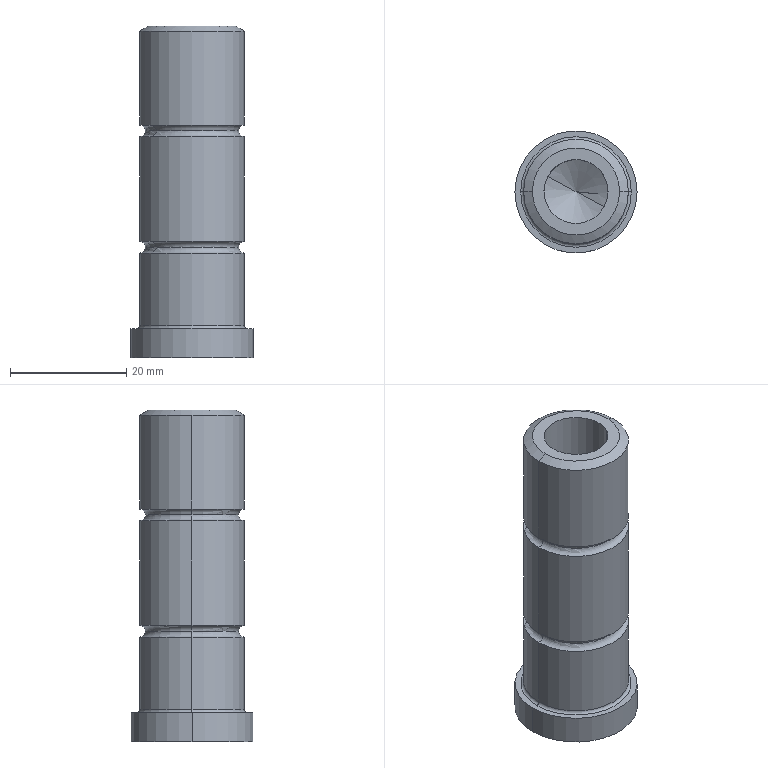Part | CATIA | 1 solid | 27 faces | box 21 x 21 x 57 mm | volume 12762 mm3 | cylinder 10 | torus 10 | cone 4 | plane 3 | commonest cylinder face diameters 18 x6 11 x2 21 x2
STEP:
#1=CARTESIAN_POINT('',(10.5,0.,-5.));
#2=VERTEX_POINT('',#1);
#3=CARTESIAN_POINT('',(-10.5,0.,-5.));
#4=VERTEX_POINT('',#3);
#5=CARTESIAN_POINT('',(0.,0.,-5.));
#6=DIRECTION('',(0.,0.,-1.));
#7=AXIS2_PLACEMENT_3D('',#5,#6,$);
#8=CIRCLE('',#7,10.5);
#9=EDGE_CURVE('',#2,#4,#8,.T.);
#10=ORIENTED_EDGE('',*,*,#9,.T.);
#11=CARTESIAN_POINT('',(0.,0.,-5.));
#12=DIRECTION('',(0.,0.,-1.));
#13=AXIS2_PLACEMENT_3D('',#11,#12,$);
#14=CIRCLE('',#13,10.5);
#15=EDGE_CURVE('',#4,#2,#14,.T.);
#16=ORIENTED_EDGE('',*,*,#15,.T.);
#17=EDGE_LOOP('',(#10,#16));
#18=FACE_OUTER_BOUND('',#17,.T.);
#19=CARTESIAN_POINT('',(0.,0.,-5.));
#20=DIRECTION('',(0.,0.,-1.));
#21=DIRECTION('',(1.,0.,0.));
#22=AXIS2_PLACEMENT_3D('',#19,#20,#21);
#23=PLANE('',#22);
#24=ADVANCED_FACE('',(#18),#23,.T.);
#25=CARTESIAN_POINT('',(-10.5,0.,0.));
#26=VERTEX_POINT('',#25);
#27=CARTESIAN_POINT('',(-10.5,0.,-2.5));
#28=DIRECTION('',(0.,0.,-1.));
#29=VECTOR('',#28,1.);
#30=LINE('',#27,#29);
#31=EDGE_CURVE('',#26,#4,#30,.T.);
#32=ORIENTED_EDGE('',*,*,#31,.F.);
#33=CARTESIAN_POINT('',(10.5,0.,0.));
#34=VERTEX_POINT('',#33);
#35=CARTESIAN_POINT('',(0.,0.,0.));
#36=DIRECTION('',(0.,0.,-1.));
#37=AXIS2_PLACEMENT_3D('',#35,#36,$);
#38=CIRCLE('',#37,10.5);
#39=EDGE_CURVE('',#26,#34,#38,.T.);
#40=ORIENTED_EDGE('',*,*,#39,.T.);
#41=CARTESIAN_POINT('',(10.5,0.,-2.5));
#42=DIRECTION('',(0.,0.,-1.));
#43=VECTOR('',#42,1.);
#44=LINE('',#41,#43);
#45=EDGE_CURVE('',#34,#2,#44,.T.);
#46=ORIENTED_EDGE('',*,*,#45,.T.);
#47=ORIENTED_EDGE('',*,*,#15,.F.);
#48=EDGE_LOOP('',(#32,#40,#46,#47));
#49=FACE_OUTER_BOUND('',#48,.T.);
#50=CARTESIAN_POINT('',(0.,0.,-2.5));
#51=DIRECTION('',(0.,0.,-1.));
#52=DIRECTION('',(1.,0.,0.));
#53=AXIS2_PLACEMENT_3D('',#50,#51,#52);
#54=CYLINDRICAL_SURFACE('',#53,10.5);
#55=ADVANCED_FACE('',(#49),#54,.T.);
#56=ORIENTED_EDGE('',*,*,#45,.F.);
#57=CARTESIAN_POINT('',(0.,0.,0.));
#58=DIRECTION('',(0.,0.,-1.));
#59=AXIS2_PLACEMENT_3D('',#57,#58,$);
#60=CIRCLE('',#59,10.5);
#61=EDGE_CURVE('',#34,#26,#60,.T.);
#62=ORIENTED_EDGE('',*,*,#61,.T.);
#63=ORIENTED_EDGE('',*,*,#31,.T.);
#64=ORIENTED_EDGE('',*,*,#9,.F.);
#65=EDGE_LOOP('',(#56,#62,#63,#64));
#66=FACE_OUTER_BOUND('',#65,.T.);
#67=ADVANCED_FACE('',(#66),#54,.T.);
#68=CARTESIAN_POINT('',(0.,0.,28.825));
#69=VERTEX_POINT('',#68);
#70=CARTESIAN_POINT('',(-4.827,2.637,32.));
#71=VERTEX_POINT('',#70);
#72=CARTESIAN_POINT('',(-2.413,1.318,30.412));
#73=DIRECTION('',(-0.76,0.4152,0.5));
#74=VECTOR('',#73,1.);
#75=LINE('',#72,#74);
#76=EDGE_CURVE('',#69,#71,#75,.T.);
#77=ORIENTED_EDGE('',*,*,#76,.T.);
#78=CARTESIAN_POINT('',(4.827,-2.637,32.));
#79=VERTEX_POINT('',#78);
#80=CARTESIAN_POINT('',(0.,0.,32.));
#81=DIRECTION('',(0.,0.,1.));
#82=AXIS2_PLACEMENT_3D('',#80,#81,$);
#83=CIRCLE('',#82,5.5);
#84=EDGE_CURVE('',#79,#71,#83,.F.);
#85=ORIENTED_EDGE('',*,*,#84,.F.);
#86=CARTESIAN_POINT('',(2.413,-1.318,30.412));
#87=DIRECTION('',(0.76,-0.4152,0.5));
#88=VECTOR('',#87,1.);
#89=LINE('',#86,#88);
#90=EDGE_CURVE('',#69,#79,#89,.T.);
#91=ORIENTED_EDGE('',*,*,#90,.F.);
#92=EDGE_LOOP('',(#77,#85,#91));
#93=FACE_OUTER_BOUND('',#92,.T.);
#94=CARTESIAN_POINT('',(0.,0.,28.825));
#95=DIRECTION('',(0.,0.,1.));
#96=DIRECTION('',(0.8776,-0.4794,0.));
#97=AXIS2_PLACEMENT_3D('',#94,#95,#96);
#98=CONICAL_SURFACE('',#97,0.,1.047);
#99=ADVANCED_FACE('',(#93),#98,.F.);
#100=ORIENTED_EDGE('',*,*,#90,.T.);
#101=CARTESIAN_POINT('',(0.,0.,32.));
#102=DIRECTION('',(0.,0.,1.));
#103=AXIS2_PLACEMENT_3D('',#101,#102,$);
#104=CIRCLE('',#103,5.5);
#105=EDGE_CURVE('',#71,#79,#104,.F.);
#106=ORIENTED_EDGE('',*,*,#105,.F.);
#107=ORIENTED_EDGE('',*,*,#76,.F.);
#108=EDGE_LOOP('',(#100,#106,#107));
#109=FACE_OUTER_BOUND('',#108,.T.);
#110=ADVANCED_FACE('',(#109),#98,.F.);
#111=CARTESIAN_POINT('',(-4.827,2.637,52.));
#112=VERTEX_POINT('',#111);
#113=CARTESIAN_POINT('',(4.827,-2.637,52.));
#114=VERTEX_POINT('',#113);
#115=CARTESIAN_POINT('',(0.,0.,52.));
#116=DIRECTION('',(0.,0.,-1.));
#117=AXIS2_PLACEMENT_3D('',#115,#116,$);
#118=CIRCLE('',#117,5.5);
#119=EDGE_CURVE('',#112,#114,#118,.F.);
#120=ORIENTED_EDGE('',*,*,#119,.T.);
#121=CARTESIAN_POINT('',(4.827,-2.637,42.155));
#122=DIRECTION('',(0.,0.,-1.));
#123=VECTOR('',#122,1.);
#124=LINE('',#121,#123);
#125=EDGE_CURVE('',#79,#114,#124,.F.);
#126=ORIENTED_EDGE('',*,*,#125,.F.);
#127=ORIENTED_EDGE('',*,*,#84,.T.);
#128=CARTESIAN_POINT('',(-4.827,2.637,42.155));
#129=DIRECTION('',(0.,0.,-1.));
#130=VECTOR('',#129,1.);
#131=LINE('',#128,#130);
#132=EDGE_CURVE('',#71,#112,#131,.F.);
#133=ORIENTED_EDGE('',*,*,#132,.T.);
#134=EDGE_LOOP('',(#120,#126,#127,#133));
#135=FACE_OUTER_BOUND('',#134,.T.);
#136=CARTESIAN_POINT('',(0.,0.,51.9));
#137=DIRECTION('',(0.,0.,-1.));
#138=DIRECTION('',(0.8776,-0.4794,0.));
#139=AXIS2_PLACEMENT_3D('',#136,#137,#138);
#140=CYLINDRICAL_SURFACE('',#139,5.5);
#141=ADVANCED_FACE('',(#135),#140,.F.);
#142=CARTESIAN_POINT('',(0.,0.,52.));
#143=DIRECTION('',(0.,0.,-1.));
#144=AXIS2_PLACEMENT_3D('',#142,#143,$);
#145=CIRCLE('',#144,5.5);
#146=EDGE_CURVE('',#114,#112,#145,.F.);
#147=ORIENTED_EDGE('',*,*,#146,.T.);
#148=ORIENTED_EDGE('',*,*,#132,.F.);
#149=ORIENTED_EDGE('',*,*,#105,.T.);
#150=ORIENTED_EDGE('',*,*,#125,.T.);
#151=EDGE_LOOP('',(#147,#148,#149,#150));
#152=FACE_OUTER_BOUND('',#151,.T.);
#153=ADVANCED_FACE('',(#152),#140,.F.);
#154=CARTESIAN_POINT('',(-7.5,0.000000168,52.));
#155=VERTEX_POINT('',#154);
#156=CARTESIAN_POINT('',(7.5,0.,52.));
#157=VERTEX_POINT('',#156);
#158=CARTESIAN_POINT('',(0.,0.,52.));
#159=DIRECTION('',(0.,0.,1.));
#160=AXIS2_PLACEMENT_3D('',#158,#159,$);
#161=CIRCLE('',#160,7.5);
#162=EDGE_CURVE('',#155,#157,#161,.T.);
#163=ORIENTED_EDGE('',*,*,#162,.T.);
#164=CARTESIAN_POINT('',(0.,0.,52.));
#165=DIRECTION('',(0.,0.,1.));
#166=AXIS2_PLACEMENT_3D('',#164,#165,$);
#167=CIRCLE('',#166,7.5);
#168=EDGE_CURVE('',#157,#155,#167,.T.);
#169=ORIENTED_EDGE('',*,*,#168,.T.);
#170=EDGE_LOOP('',(#163,#169));
#171=FACE_OUTER_BOUND('',#170,.T.);
#172=ORIENTED_EDGE('',*,*,#119,.F.);
#173=ORIENTED_EDGE('',*,*,#146,.F.);
#174=EDGE_LOOP('',(#172,#173));
#175=FACE_BOUND('',#174,.T.);
#176=CARTESIAN_POINT('',(0.,0.,52.));
#177=DIRECTION('',(0.,0.,1.));
#178=DIRECTION('',(1.,0.,0.));
#179=AXIS2_PLACEMENT_3D('',#176,#177,#178);
#180=PLANE('',#179);
#181=ADVANCED_FACE('',(#171,#175),#180,.T.);
#182=CARTESIAN_POINT('',(-9.,0.,51.134));
#183=VERTEX_POINT('',#182);
#184=CARTESIAN_POINT('',(-8.25,0.,51.567));
#185=DIRECTION('',(-0.866,0.,-0.5));
#186=VECTOR('',#185,1.);
#187=LINE('',#184,#186);
#188=EDGE_CURVE('',#155,#183,#187,.T.);
#189=ORIENTED_EDGE('',*,*,#188,.T.);
#190=CARTESIAN_POINT('',(9.,0.,51.134));
#191=VERTEX_POINT('',#190);
#192=CARTESIAN_POINT('',(0.,0.,51.134));
#193=DIRECTION('',(0.,0.,1.));
#194=AXIS2_PLACEMENT_3D('',#192,#193,$);
#195=CIRCLE('',#194,9.);
#196=EDGE_CURVE('',#183,#191,#195,.T.);
#197=ORIENTED_EDGE('',*,*,#196,.T.);
#198=CARTESIAN_POINT('',(8.25,0.,51.567));
#199=DIRECTION('',(0.866,0.,-0.5));
#200=VECTOR('',#199,1.);
#201=LINE('',#198,#200);
#202=EDGE_CURVE('',#157,#191,#201,.T.);
#203=ORIENTED_EDGE('',*,*,#202,.F.);
#204=ORIENTED_EDGE('',*,*,#162,.F.);
#205=EDGE_LOOP('',(#189,#197,#203,#204));
#206=FACE_OUTER_BOUND('',#205,.T.);
#207=CARTESIAN_POINT('',(0.,0.,56.33));
#208=DIRECTION('',(0.,0.,-1.));
#209=DIRECTION('',(-0.894,0.4481,0.));
#210=AXIS2_PLACEMENT_3D('',#207,#208,#209);
#211=CONICAL_SURFACE('',#210,0.,1.047);
#212=ADVANCED_FACE('',(#206),#211,.T.);
#213=ORIENTED_EDGE('',*,*,#202,.T.);
#214=CARTESIAN_POINT('',(0.,0.,51.134));
#215=DIRECTION('',(0.,0.,1.));
#216=AXIS2_PLACEMENT_3D('',#214,#215,$);
#217=CIRCLE('',#216,9.);
#218=EDGE_CURVE('',#191,#183,#217,.T.);
#219=ORIENTED_EDGE('',*,*,#218,.T.);
#220=ORIENTED_EDGE('',*,*,#188,.F.);
#221=ORIENTED_EDGE('',*,*,#168,.F.);
#222=EDGE_LOOP('',(#213,#219,#220,#221));
#223=FACE_OUTER_BOUND('',#222,.T.);
#224=CARTESIAN_POINT('',(0.,0.,56.33));
#225=DIRECTION('',(0.,0.,-1.));
#226=DIRECTION('',(1.,0.,0.));
#227=AXIS2_PLACEMENT_3D('',#224,#225,#226);
#228=CONICAL_SURFACE('',#227,0.,1.047);
#229=ADVANCED_FACE('',(#223),#228,.T.);
#230=ORIENTED_EDGE('',*,*,#39,.F.);
#231=ORIENTED_EDGE('',*,*,#61,.F.);
#232=EDGE_LOOP('',(#230,#231));
#233=FACE_OUTER_BOUND('',#232,.T.);
#234=CARTESIAN_POINT('',(9.5,0.,0.));
#235=VERTEX_POINT('',#234);
#236=CARTESIAN_POINT('',(-9.5,-0.000000008,0.));
#237=VERTEX_POINT('',#236);
#238=CARTESIAN_POINT('',(0.,0.,0.));
#239=DIRECTION('',(0.,0.,1.));
#240=AXIS2_PLACEMENT_3D('',#238,#239,$);
#241=CIRCLE('',#240,9.5);
#242=EDGE_CURVE('',#235,#237,#241,.F.);
#243=ORIENTED_EDGE('',*,*,#242,.T.);
#244=CARTESIAN_POINT('',(0.,0.,0.));
#245=DIRECTION('',(0.,0.,1.));
#246=AXIS2_PLACEMENT_3D('',#244,#245,$);
#247=CIRCLE('',#246,9.5);
#248=EDGE_CURVE('',#237,#235,#247,.F.);
#249=ORIENTED_EDGE('',*,*,#248,.T.);
#250=EDGE_LOOP('',(#243,#249));
#251=FACE_BOUND('',#250,.T.);
#252=CARTESIAN_POINT('',(0.,0.,0.));
#253=DIRECTION('',(0.,0.,1.));
#254=DIRECTION('',(1.,0.,0.));
#255=AXIS2_PLACEMENT_3D('',#252,#253,#254);
#256=PLANE('',#255);
#257=ADVANCED_FACE('',(#233,#251),#256,.T.);
#258=CARTESIAN_POINT('',(-9.,0.,0.5));
#259=VERTEX_POINT('',#258);
#260=CARTESIAN_POINT('',(9.,0.,0.5));
#261=VERTEX_POINT('',#260);
#262=CARTESIAN_POINT('',(0.,0.,0.5));
#263=DIRECTION('',(0.,0.,1.));
#264=AXIS2_PLACEMENT_3D('',#262,#263,$);
#265=CIRCLE('',#264,9.);
#266=EDGE_CURVE('',#259,#261,#265,.F.);
#267=ORIENTED_EDGE('',*,*,#266,.T.);
#268=CARTESIAN_POINT('',(9.5,0.,0.5));
#269=DIRECTION('',(0.,-1.,0.));
#270=AXIS2_PLACEMENT_3D('',#268,#269,$);
#271=CIRCLE('',#270,0.5);
#272=EDGE_CURVE('',#261,#235,#271,.T.);
#273=ORIENTED_EDGE('',*,*,#272,.T.);
#274=ORIENTED_EDGE('',*,*,#248,.F.);
#275=CARTESIAN_POINT('',(-9.5,0.000000067,0.5));
#276=DIRECTION('',(0.000000007,1.,0.));
#277=AXIS2_PLACEMENT_3D('',#275,#276,$);
#278=CIRCLE('',#277,0.5);
#279=EDGE_CURVE('',#259,#237,#278,.T.);
#280=ORIENTED_EDGE('',*,*,#279,.F.);
#281=EDGE_LOOP('',(#267,#273,#274,#280));
#282=FACE_OUTER_BOUND('',#281,.T.);
#283=CARTESIAN_POINT('',(0.,0.,0.5));
#284=DIRECTION('',(0.,0.,1.));
#285=DIRECTION('',(1.,0.,0.));
#286=AXIS2_PLACEMENT_3D('',#283,#284,#285);
#287=TOROIDAL_SURFACE('',#286,9.5,0.5);
#288=ADVANCED_FACE('',(#282),#287,.F.);
#289=CARTESIAN_POINT('',(0.,0.,0.5));
#290=DIRECTION('',(0.,0.,1.));
#291=AXIS2_PLACEMENT_3D('',#289,#290,$);
#292=CIRCLE('',#291,9.);
#293=EDGE_CURVE('',#261,#259,#292,.F.);
#294=ORIENTED_EDGE('',*,*,#293,.T.);
#295=ORIENTED_EDGE('',*,*,#279,.T.);
#296=ORIENTED_EDGE('',*,*,#242,.F.);
#297=ORIENTED_EDGE('',*,*,#272,.F.);
#298=EDGE_LOOP('',(#294,#295,#296,#297));
#299=FACE_OUTER_BOUND('',#298,.T.);
#300=CARTESIAN_POINT('',(0.,0.,0.5));
#301=DIRECTION('',(0.,0.,1.));
#302=DIRECTION('',(-0.9997,0.02353,0.));
#303=AXIS2_PLACEMENT_3D('',#300,#301,#302);
#304=TOROIDAL_SURFACE('',#303,9.5,0.5);
#305=ADVANCED_FACE('',(#299),#304,.F.);
#306=CARTESIAN_POINT('',(-9.,0.000000203,15.));
#307=VERTEX_POINT('',#306);
#308=CARTESIAN_POINT('',(-9.,0.,33.));
#309=VERTEX_POINT('',#308);
#310=CARTESIAN_POINT('',(-9.,0.,26.));
#311=DIRECTION('',(0.,0.,1.));
#312=VECTOR('',#311,1.);
#313=LINE('',#310,#312);
#314=EDGE_CURVE('',#307,#309,#313,.T.);
#315=ORIENTED_EDGE('',*,*,#314,.T.);
#316=CARTESIAN_POINT('',(9.,0.,33.));
#317=VERTEX_POINT('',#316);
#318=CARTESIAN_POINT('',(0.,0.,33.));
#319=DIRECTION('',(0.,0.,1.));
#320=AXIS2_PLACEMENT_3D('',#318,#319,$);
#321=CIRCLE('',#320,9.);
#322=EDGE_CURVE('',#317,#309,#321,.T.);
#323=ORIENTED_EDGE('',*,*,#322,.F.);
#324=CARTESIAN_POINT('',(9.,-0.000000009,15.));
#325=VERTEX_POINT('',#324);
#326=CARTESIAN_POINT('',(9.,0.,26.));
#327=DIRECTION('',(0.,0.,1.));
#328=VECTOR('',#327,1.);
#329=LINE('',#326,#328);
#330=EDGE_CURVE('',#325,#317,#329,.T.);
#331=ORIENTED_EDGE('',*,*,#330,.F.);
#332=CARTESIAN_POINT('',(0.,0.,15.));
#333=DIRECTION('',(0.,0.,1.));
#334=AXIS2_PLACEMENT_3D('',#332,#333,$);
#335=CIRCLE('',#334,9.);
#336=EDGE_CURVE('',#325,#307,#335,.T.);
#337=ORIENTED_EDGE('',*,*,#336,.T.);
#338=EDGE_LOOP('',(#315,#323,#331,#337));
#339=FACE_OUTER_BOUND('',#338,.T.);
#340=CARTESIAN_POINT('',(0.,0.,26.));
#341=DIRECTION('',(0.,0.,1.));
#342=DIRECTION('',(1.,0.,0.));
#343=AXIS2_PLACEMENT_3D('',#340,#341,#342);
#344=CYLINDRICAL_SURFACE('',#343,9.);
#345=ADVANCED_FACE('',(#339),#344,.T.);
#346=CARTESIAN_POINT('',(9.,0.,13.));
#347=VERTEX_POINT('',#346);
#348=CARTESIAN_POINT('',(9.,0.,26.));
#349=DIRECTION('',(0.,0.,1.));
#350=VECTOR('',#349,1.);
#351=LINE('',#348,#350);
#352=EDGE_CURVE('',#261,#347,#351,.T.);
#353=ORIENTED_EDGE('',*,*,#352,.F.);
#354=ORIENTED_EDGE('',*,*,#266,.F.);
#355=CARTESIAN_POINT('',(-9.,0.,13.));
#356=VERTEX_POINT('',#355);
#357=CARTESIAN_POINT('',(-9.,0.,26.));
#358=DIRECTION('',(0.,0.,1.));
#359=VECTOR('',#358,1.);
#360=LINE('',#357,#359);
#361=EDGE_CURVE('',#259,#356,#360,.T.);
#362=ORIENTED_EDGE('',*,*,#361,.T.);
#363=CARTESIAN_POINT('',(0.,0.,13.));
#364=DIRECTION('',(0.,0.,1.));
#365=AXIS2_PLACEMENT_3D('',#363,#364,$);
#366=CIRCLE('',#365,9.);
#367=EDGE_CURVE('',#347,#356,#366,.T.);
#368=ORIENTED_EDGE('',*,*,#367,.F.);
#369=EDGE_LOOP('',(#353,#354,#362,#368));
#370=FACE_OUTER_BOUND('',#369,.T.);
#371=ADVANCED_FACE('',(#370),#344,.T.);
#372=CARTESIAN_POINT('',(-9.,0.,35.));
#373=VERTEX_POINT('',#372);
#374=CARTESIAN_POINT('',(-9.,0.,26.));
#375=DIRECTION('',(0.,0.,1.));
#376=VECTOR('',#375,1.);
#377=LINE('',#374,#376);
#378=EDGE_CURVE('',#373,#183,#377,.T.);
#379=ORIENTED_EDGE('',*,*,#378,.T.);
#380=ORIENTED_EDGE('',*,*,#218,.F.);
#381=CARTESIAN_POINT('',(9.,-0.000000009,35.));
#382=VERTEX_POINT('',#381);
#383=CARTESIAN_POINT('',(9.,0.,26.));
#384=DIRECTION('',(0.,0.,1.));
#385=VECTOR('',#384,1.);
#386=LINE('',#383,#385);
#387=EDGE_CURVE('',#382,#191,#386,.T.);
#388=ORIENTED_EDGE('',*,*,#387,.F.);
#389=CARTESIAN_POINT('',(0.,0.,35.));
#390=DIRECTION('',(0.,0.,1.));
#391=AXIS2_PLACEMENT_3D('',#389,#390,$);
#392=CIRCLE('',#391,9.);
#393=EDGE_CURVE('',#382,#373,#392,.T.);
#394=ORIENTED_EDGE('',*,*,#393,.T.);
#395=EDGE_LOOP('',(#379,#380,#388,#394));
#396=FACE_OUTER_BOUND('',#395,.T.);
#397=ADVANCED_FACE('',(#396),#344,.T.);
#398=ORIENTED_EDGE('',*,*,#330,.T.);
#399=CARTESIAN_POINT('',(0.,0.,33.));
#400=DIRECTION('',(0.,0.,1.));
#401=AXIS2_PLACEMENT_3D('',#399,#400,$);
#402=CIRCLE('',#401,9.);
#403=EDGE_CURVE('',#309,#317,#402,.T.);
#404=ORIENTED_EDGE('',*,*,#403,.F.);
#405=ORIENTED_EDGE('',*,*,#314,.F.);
#406=CARTESIAN_POINT('',(0.,0.,15.));
#407=DIRECTION('',(0.,0.,1.));
#408=AXIS2_PLACEMENT_3D('',#406,#407,$);
#409=CIRCLE('',#408,9.);
#410=EDGE_CURVE('',#307,#325,#409,.T.);
#411=ORIENTED_EDGE('',*,*,#410,.T.);
#412=EDGE_LOOP('',(#398,#404,#405,#411));
#413=FACE_OUTER_BOUND('',#412,.T.);
#414=ADVANCED_FACE('',(#413),#344,.T.);
#415=ORIENTED_EDGE('',*,*,#361,.F.);
#416=ORIENTED_EDGE('',*,*,#293,.F.);
#417=ORIENTED_EDGE('',*,*,#352,.T.);
#418=CARTESIAN_POINT('',(0.,0.,13.));
#419=DIRECTION('',(0.,0.,1.));
#420=AXIS2_PLACEMENT_3D('',#418,#419,$);
#421=CIRCLE('',#420,9.);
#422=EDGE_CURVE('',#356,#347,#421,.T.);
#423=ORIENTED_EDGE('',*,*,#422,.F.);
#424=EDGE_LOOP('',(#415,#416,#417,#423));
#425=FACE_OUTER_BOUND('',#424,.T.);
#426=ADVANCED_FACE('',(#425),#344,.T.);
#427=ORIENTED_EDGE('',*,*,#387,.T.);
#428=ORIENTED_EDGE('',*,*,#196,.F.);
#429=ORIENTED_EDGE('',*,*,#378,.F.);
#430=CARTESIAN_POINT('',(0.,0.,35.));
#431=DIRECTION('',(0.,0.,1.));
#432=AXIS2_PLACEMENT_3D('',#430,#431,$);
#433=CIRCLE('',#432,9.);
#434=EDGE_CURVE('',#373,#382,#433,.T.);
#435=ORIENTED_EDGE('',*,*,#434,.T.);
#436=EDGE_LOOP('',(#427,#428,#429,#435));
#437=FACE_OUTER_BOUND('',#436,.T.);
#438=ADVANCED_FACE('',(#437),#344,.T.);
#439=CARTESIAN_POINT('',(-8.,0.,34.));
#440=VERTEX_POINT('',#439);
#441=CARTESIAN_POINT('',(8.,0.,34.));
#442=VERTEX_POINT('',#441);
#443=CARTESIAN_POINT('',(0.,0.,34.));
#444=DIRECTION('',(0.,0.,1.));
#445=AXIS2_PLACEMENT_3D('',#443,#444,$);
#446=CIRCLE('',#445,8.);
#447=EDGE_CURVE('',#440,#442,#446,.T.);
#448=ORIENTED_EDGE('',*,*,#447,.T.);
#449=CARTESIAN_POINT('',(9.,-0.000000009,34.));
#450=DIRECTION('',(-0.000000001,-1.,0.));
#451=AXIS2_PLACEMENT_3D('',#449,#450,$);
#452=CIRCLE('',#451,1.);
#453=EDGE_CURVE('',#442,#382,#452,.F.);
#454=ORIENTED_EDGE('',*,*,#453,.T.);
#455=ORIENTED_EDGE('',*,*,#434,.F.);
#456=CARTESIAN_POINT('',(-9.,0.000000203,34.));
#457=DIRECTION('',(0.000000023,1.,0.));
#458=AXIS2_PLACEMENT_3D('',#456,#457,$);
#459=CIRCLE('',#458,1.);
#460=EDGE_CURVE('',#440,#373,#459,.F.);
#461=ORIENTED_EDGE('',*,*,#460,.F.);
#462=EDGE_LOOP('',(#448,#454,#455,#461));
#463=FACE_OUTER_BOUND('',#462,.T.);
#464=CARTESIAN_POINT('',(0.,0.,34.));
#465=DIRECTION('',(0.,0.,1.));
#466=DIRECTION('',(-0.9911,0.1331,0.));
#467=AXIS2_PLACEMENT_3D('',#464,#465,#466);
#468=TOROIDAL_SURFACE('',#467,9.,1.);
#469=ADVANCED_FACE('',(#463),#468,.F.);
#470=CARTESIAN_POINT('',(0.,0.,34.));
#471=DIRECTION('',(0.,0.,1.));
#472=AXIS2_PLACEMENT_3D('',#470,#471,$);
#473=CIRCLE('',#472,8.);
#474=EDGE_CURVE('',#442,#440,#473,.T.);
#475=ORIENTED_EDGE('',*,*,#474,.T.);
#476=ORIENTED_EDGE('',*,*,#460,.T.);
#477=ORIENTED_EDGE('',*,*,#393,.F.);
#478=ORIENTED_EDGE('',*,*,#453,.F.);
#479=EDGE_LOOP('',(#475,#476,#477,#478));
#480=FACE_OUTER_BOUND('',#479,.T.);
#481=CARTESIAN_POINT('',(0.,0.,34.));
#482=DIRECTION('',(0.,0.,1.));
#483=DIRECTION('',(0.9881,-0.154,0.));
#484=AXIS2_PLACEMENT_3D('',#481,#482,#483);
#485=TOROIDAL_SURFACE('',#484,9.,1.);
#486=ADVANCED_FACE('',(#480),#485,.F.);
#487=ORIENTED_EDGE('',*,*,#403,.T.);
#488=CARTESIAN_POINT('',(9.,0.,34.));
#489=DIRECTION('',(0.,-1.,0.));
#490=AXIS2_PLACEMENT_3D('',#488,#489,$);
#491=CIRCLE('',#490,1.);
#492=EDGE_CURVE('',#317,#442,#491,.F.);
#493=ORIENTED_EDGE('',*,*,#492,.T.);
#494=ORIENTED_EDGE('',*,*,#447,.F.);
#495=CARTESIAN_POINT('',(-9.,0.,34.));
#496=DIRECTION('',(0.,1.,0.));
#497=AXIS2_PLACEMENT_3D('',#495,#496,$);
#498=CIRCLE('',#497,1.);
#499=EDGE_CURVE('',#309,#440,#498,.F.);
#500=ORIENTED_EDGE('',*,*,#499,.F.);
#501=EDGE_LOOP('',(#487,#493,#494,#500));
#502=FACE_OUTER_BOUND('',#501,.T.);
#503=CARTESIAN_POINT('',(0.,0.,34.));
#504=DIRECTION('',(0.,0.,1.));
#505=DIRECTION('',(-0.9033,0.4291,0.));
#506=AXIS2_PLACEMENT_3D('',#503,#504,#505);
#507=TOROIDAL_SURFACE('',#506,9.,1.);
#508=ADVANCED_FACE('',(#502),#507,.F.);
#509=ORIENTED_EDGE('',*,*,#322,.T.);
#510=ORIENTED_EDGE('',*,*,#499,.T.);
#511=ORIENTED_EDGE('',*,*,#474,.F.);
#512=ORIENTED_EDGE('',*,*,#492,.F.);
#513=EDGE_LOOP('',(#509,#510,#511,#512));
#514=FACE_OUTER_BOUND('',#513,.T.);
#515=CARTESIAN_POINT('',(0.,0.,34.));
#516=DIRECTION('',(0.,0.,1.));
#517=DIRECTION('',(0.894,-0.448,0.));
#518=AXIS2_PLACEMENT_3D('',#515,#516,#517);
#519=TOROIDAL_SURFACE('',#518,9.,1.);
#520=ADVANCED_FACE('',(#514),#519,.F.);
#521=CARTESIAN_POINT('',(-8.,0.,14.));
#522=VERTEX_POINT('',#521);
#523=CARTESIAN_POINT('',(8.,0.,14.));
#524=VERTEX_POINT('',#523);
#525=CARTESIAN_POINT('',(0.,0.,14.));
#526=DIRECTION('',(0.,0.,1.));
#527=AXIS2_PLACEMENT_3D('',#525,#526,$);
#528=CIRCLE('',#527,8.);
#529=EDGE_CURVE('',#522,#524,#528,.T.);
#530=ORIENTED_EDGE('',*,*,#529,.T.);
#531=CARTESIAN_POINT('',(9.,-0.000000009,14.));
#532=DIRECTION('',(-0.000000001,-1.,0.));
#533=AXIS2_PLACEMENT_3D('',#531,#532,$);
#534=CIRCLE('',#533,1.);
#535=EDGE_CURVE('',#524,#325,#534,.F.);
#536=ORIENTED_EDGE('',*,*,#535,.T.);
#537=ORIENTED_EDGE('',*,*,#410,.F.);
#538=CARTESIAN_POINT('',(-9.,0.000000203,14.));
#539=DIRECTION('',(0.000000023,1.,0.));
#540=AXIS2_PLACEMENT_3D('',#538,#539,$);
#541=CIRCLE('',#540,1.);
#542=EDGE_CURVE('',#522,#307,#541,.F.);
#543=ORIENTED_EDGE('',*,*,#542,.F.);
#544=EDGE_LOOP('',(#530,#536,#537,#543));
#545=FACE_OUTER_BOUND('',#544,.T.);
#546=CARTESIAN_POINT('',(0.,0.,14.));
#547=DIRECTION('',(0.,0.,1.));
#548=DIRECTION('',(-0.9911,0.1331,0.));
#549=AXIS2_PLACEMENT_3D('',#546,#547,#548);
#550=TOROIDAL_SURFACE('',#549,9.,1.);
#551=ADVANCED_FACE('',(#545),#550,.F.);
#552=CARTESIAN_POINT('',(0.,0.,14.));
#553=DIRECTION('',(0.,0.,1.));
#554=AXIS2_PLACEMENT_3D('',#552,#553,$);
#555=CIRCLE('',#554,8.);
#556=EDGE_CURVE('',#524,#522,#555,.T.);
#557=ORIENTED_EDGE('',*,*,#556,.T.);
#558=ORIENTED_EDGE('',*,*,#542,.T.);
#559=ORIENTED_EDGE('',*,*,#336,.F.);
#560=ORIENTED_EDGE('',*,*,#535,.F.);
#561=EDGE_LOOP('',(#557,#558,#559,#560));
#562=FACE_OUTER_BOUND('',#561,.T.);
#563=CARTESIAN_POINT('',(0.,0.,14.));
#564=DIRECTION('',(0.,0.,1.));
#565=DIRECTION('',(0.9881,-0.154,0.));
#566=AXIS2_PLACEMENT_3D('',#563,#564,#565);
#567=TOROIDAL_SURFACE('',#566,9.,1.);
#568=ADVANCED_FACE('',(#562),#567,.F.);
#569=ORIENTED_EDGE('',*,*,#422,.T.);
#570=CARTESIAN_POINT('',(9.,0.,14.));
#571=DIRECTION('',(0.,-1.,0.));
#572=AXIS2_PLACEMENT_3D('',#570,#571,$);
#573=CIRCLE('',#572,1.);
#574=EDGE_CURVE('',#347,#524,#573,.F.);
#575=ORIENTED_EDGE('',*,*,#574,.T.);
#576=ORIENTED_EDGE('',*,*,#529,.F.);
#577=CARTESIAN_POINT('',(-9.,0.,14.));
#578=DIRECTION('',(0.,1.,0.));
#579=AXIS2_PLACEMENT_3D('',#577,#578,$);
#580=CIRCLE('',#579,1.);
#581=EDGE_CURVE('',#356,#522,#580,.F.);
#582=ORIENTED_EDGE('',*,*,#581,.F.);
#583=EDGE_LOOP('',(#569,#575,#576,#582));
#584=FACE_OUTER_BOUND('',#583,.T.);
#585=CARTESIAN_POINT('',(0.,0.,14.));
#586=DIRECTION('',(0.,0.,1.));
#587=DIRECTION('',(-0.9033,0.4291,0.));
#588=AXIS2_PLACEMENT_3D('',#585,#586,#587);
#589=TOROIDAL_SURFACE('',#588,9.,1.);
#590=ADVANCED_FACE('',(#584),#589,.F.);
#591=ORIENTED_EDGE('',*,*,#367,.T.);
#592=ORIENTED_EDGE('',*,*,#581,.T.);
#593=ORIENTED_EDGE('',*,*,#556,.F.);
#594=ORIENTED_EDGE('',*,*,#574,.F.);
#595=EDGE_LOOP('',(#591,#592,#593,#594));
#596=FACE_OUTER_BOUND('',#595,.T.);
#597=CARTESIAN_POINT('',(0.,0.,14.));
#598=DIRECTION('',(0.,0.,1.));
#599=DIRECTION('',(0.894,-0.448,0.));
#600=AXIS2_PLACEMENT_3D('',#597,#598,#599);
#601=TOROIDAL_SURFACE('',#600,9.,1.);
#602=ADVANCED_FACE('',(#596),#601,.F.);
#603=CLOSED_SHELL('',(#24,#55,#67,#99,#110,#141,#153,#181,#212,#229,#257,#288,#305,#345,#371,#397,#414,#426,#438,#469,#486,#508,#520,#551,#568,#590,#602));
#604=MANIFOLD_SOLID_BREP('',#603);
#605=(LENGTH_UNIT()NAMED_UNIT(*)SI_UNIT(.MILLI.,.METRE.));
#606=UNCERTAINTY_MEASURE_WITH_UNIT(LENGTH_MEASURE(0.005),#605,'','');
#607=(NAMED_UNIT(*)PLANE_ANGLE_UNIT()SI_UNIT($,.RADIAN.));
#608=(NAMED_UNIT(*)SI_UNIT($,.STERADIAN.)SOLID_ANGLE_UNIT());
#609=(GEOMETRIC_REPRESENTATION_CONTEXT(3)GLOBAL_UNCERTAINTY_ASSIGNED_CONTEXT((#606))GLOBAL_UNIT_ASSIGNED_CONTEXT((#605,#607,#608))REPRESENTATION_CONTEXT('',''));
#610=ADVANCED_BREP_SHAPE_REPRESENTATION('',(#604),#609);